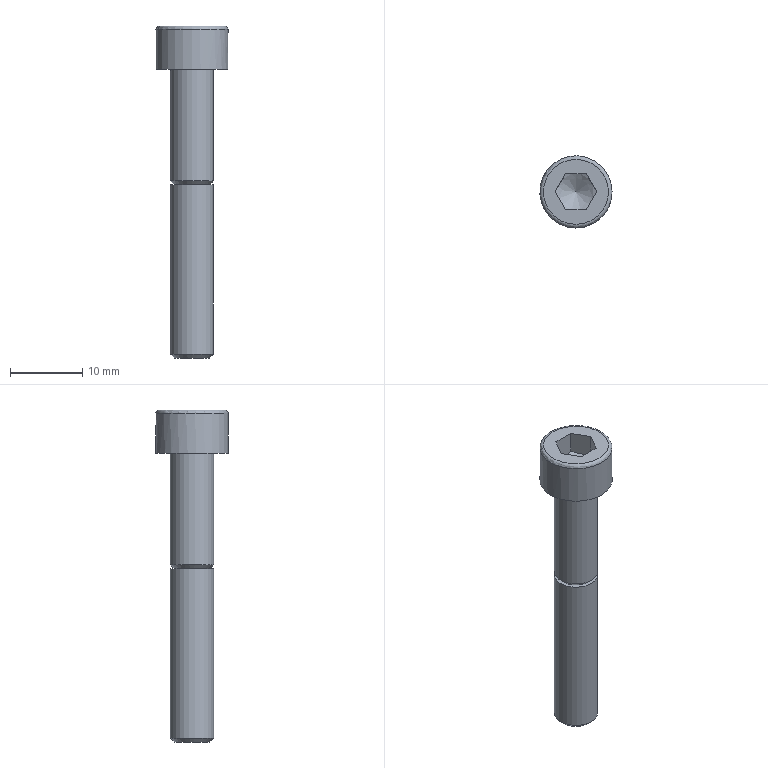Part | STEP file | 1_38 | 1 solid | 17 faces | box 10 x 10 x 46 mm | volume 1516 mm3 | plane 10 | cylinder 3 | cone 3 | torus 1 | commonest cylinder face diameters 6 x2 10 x1